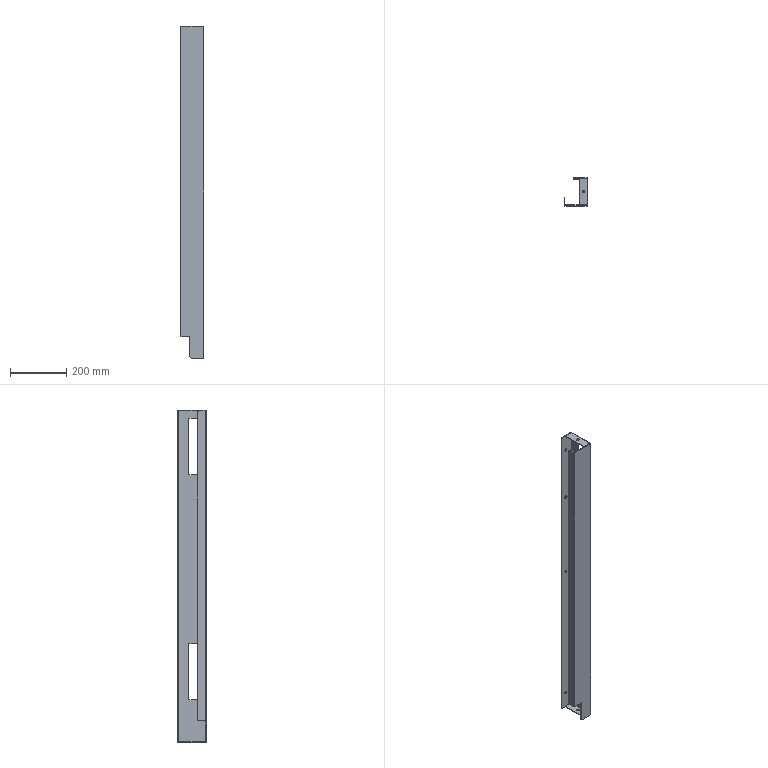Part | STEP file | HESS-408-70-15W-W-29-outer case lower support 4 | 1 solid | 77 faces | box 85 x 100 x 1180 mm | volume 851335 mm3 | plane 42 | cylinder 35 | commonest cylinder face diameters 9 x10 6 x8 0.2 x5 6.2 x5 10 x4 12 x2